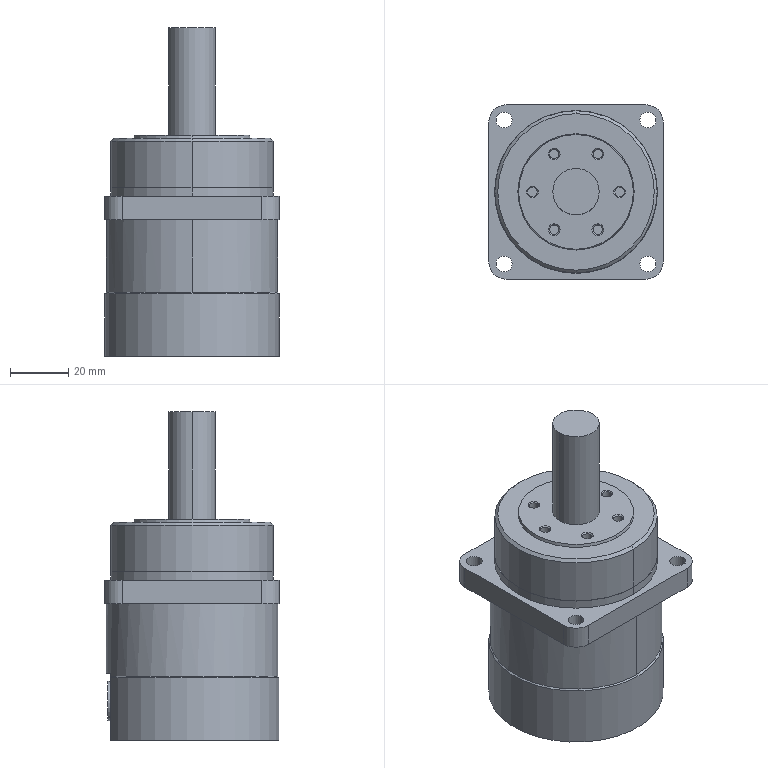Part | STEP file | PN_0007_Flange-Body201 | 1 solid | 204 faces | box 60 x 60 x 113 mm | volume 194551 mm3 | cylinder 84 | plane 81 | cone 39 | commonest cylinder face diameters 3.242 x20 5.5 x18 6.5 x11 3 x6 12 x4 30 x4